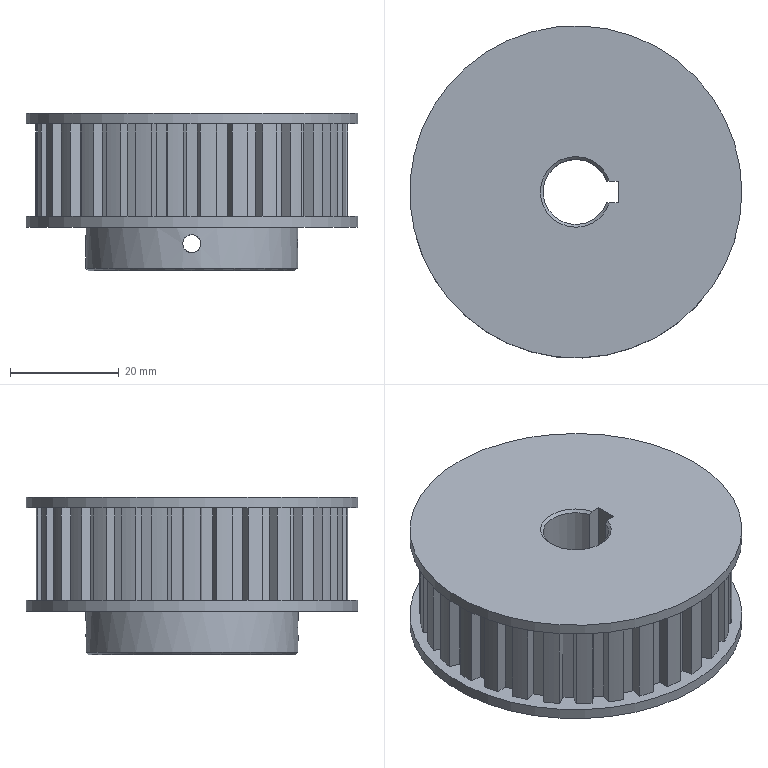Part | NX | 1 solid | 138 faces | box 61 x 61 x 29 mm | volume 58662 mm3 | plane 98 | cylinder 37 | cone 3 | commonest cylinder face diameters 57.3 x30 3.3 x3 61 x2 12 x1 39 x1